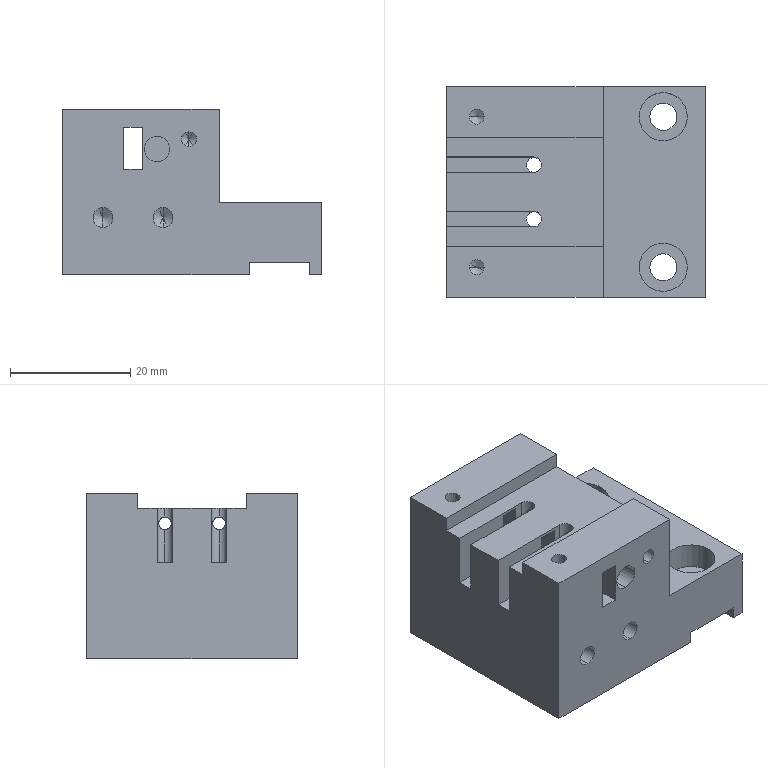Part | STEP file | D03 | 1 solid | 98 faces | box 43 x 35 x 27.5 mm | volume 27305 mm3 | cylinder 44 | plane 38 | cone 16 | commonest cylinder face diameters 2.5 x12 2.1 x8 3.3 x8 2.6 x4 4.2 x4 4.5 x4